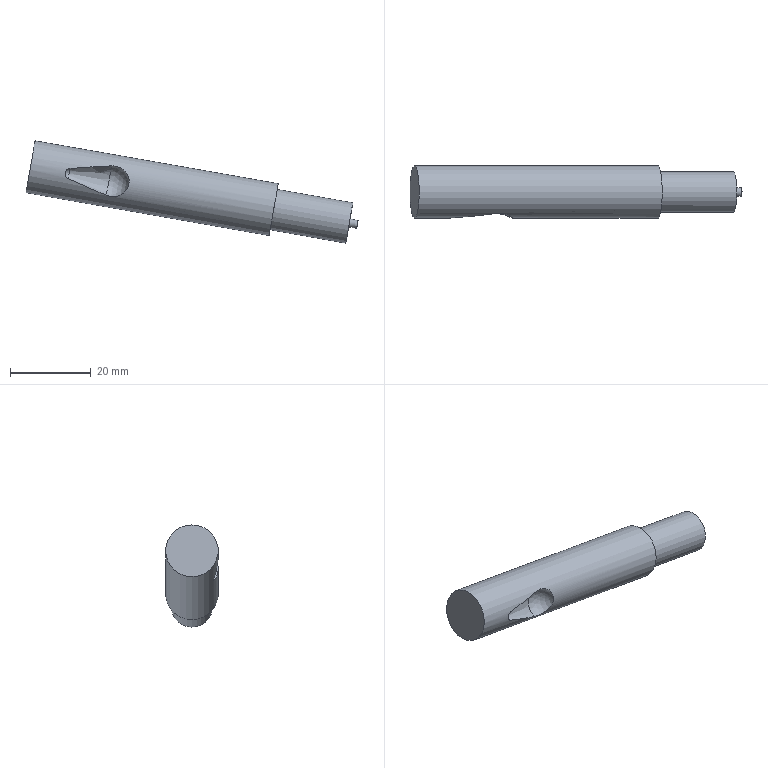Part | NX | features solid 2 | 1 solid | 10 faces | volume 9441 mm3 | plane 4 | cylinder 3 | sphere 2 | cone 1 | commonest cylinder face diameters 2 x1 10.1 x1 13 x1
STEP:
#1=CARTESIAN_POINT('',(396.16,145.871,8.418));
#2=VERTEX_POINT('',#1);
#3=CARTESIAN_POINT('',(395.283,145.871,3.444));
#4=DIRECTION('',(0.9848,0.,-0.1736));
#5=DIRECTION('',(0.1736,0.,0.9848));
#6=AXIS2_PLACEMENT_3D('',#3,#4,#5);
#7=CIRCLE('',#6,5.05);
#8=EDGE_CURVE('',#2,#2,#7,.T.);
#9=ORIENTED_EDGE('',*,*,#8,.T.);
#10=EDGE_LOOP('',(#9));
#11=FACE_BOUND('',#10,.T.);
#12=CARTESIAN_POINT('',(395.456,145.871,4.429));
#13=VERTEX_POINT('',#12);
#14=CARTESIAN_POINT('',(395.283,145.871,3.444));
#15=DIRECTION('',(0.9848,0.,-0.1736));
#16=DIRECTION('',(0.1736,0.,0.9848));
#17=AXIS2_PLACEMENT_3D('',#14,#15,#16);
#18=CIRCLE('',#17,1.);
#19=EDGE_CURVE('',#13,#13,#18,.F.);
#20=ORIENTED_EDGE('',*,*,#19,.T.);
#21=EDGE_LOOP('',(#20));
#22=FACE_BOUND('',#21,.T.);
#23=CARTESIAN_POINT('',(395.283,145.871,3.444));
#24=DIRECTION('',(-0.9848,0.,0.1736));
#25=DIRECTION('',(0.1736,0.,0.9848));
#26=AXIS2_PLACEMENT_3D('',#23,#24,#25);
#27=PLANE('',#26);
#28=ADVANCED_FACE('',(#11,#22),#27,.F.);
#29=CARTESIAN_POINT('',(336.508,140.525,17.562));
#30=VERTEX_POINT('',#29);
#31=CARTESIAN_POINT('',(326.241,139.499,16.923));
#32=VERTEX_POINT('',#31);
#33=CARTESIAN_POINT('',(336.508,140.525,17.562));
#34=CARTESIAN_POINT('',(333.101,140.013,17.411));
#35=CARTESIAN_POINT('',(329.675,139.671,17.179));
#36=CARTESIAN_POINT('',(326.241,139.499,16.923));
#37=B_SPLINE_CURVE_WITH_KNOTS('',3,(#33,#34,#35,#36),.UNSPECIFIED.,.F.,.F.,(4,4),(0.000000207,0.01034),.UNSPECIFIED.);
#38=EDGE_CURVE('',#30,#32,#37,.T.);
#39=ORIENTED_EDGE('',*,*,#38,.F.);
#40=CARTESIAN_POINT('',(335.224,140.525,10.28));
#41=VERTEX_POINT('',#40);
#42=CARTESIAN_POINT('',(335.224,140.525,10.28));
#43=CARTESIAN_POINT('',(336.35,140.708,9.813));
#44=CARTESIAN_POINT('',(338.335,140.377,9.801));
#45=CARTESIAN_POINT('',(340.189,139.555,11.301));
#46=CARTESIAN_POINT('',(340.929,139.279,13.019));
#47=CARTESIAN_POINT('',(340.826,139.556,14.903));
#48=CARTESIAN_POINT('',(339.907,140.159,16.431));
#49=CARTESIAN_POINT('',(338.355,140.634,17.394));
#50=CARTESIAN_POINT('',(337.117,140.617,17.589));
#51=CARTESIAN_POINT('',(336.508,140.525,17.562));
#52=B_SPLINE_CURVE_WITH_KNOTS('',3,(#42,#43,#44,#45,#46,#47,#48,#49,#50,#51),.UNSPECIFIED.,.F.,.F.,(4,1,1,1,1,1,1,4),(0.000000204,0.003647,0.005471,0.007295,0.009118,0.01094,0.01277,0.01459),.UNSPECIFIED.);
#53=EDGE_CURVE('',#41,#30,#52,.T.);
#54=ORIENTED_EDGE('',*,*,#53,.F.);
#55=CARTESIAN_POINT('',(325.795,139.499,14.393));
#56=VERTEX_POINT('',#55);
#57=CARTESIAN_POINT('',(325.795,139.499,14.393));
#58=CARTESIAN_POINT('',(328.935,139.671,12.977));
#59=CARTESIAN_POINT('',(332.073,140.013,11.588));
#60=CARTESIAN_POINT('',(335.224,140.525,10.28));
#61=B_SPLINE_CURVE_WITH_KNOTS('',3,(#57,#58,#59,#60),.UNSPECIFIED.,.F.,.F.,(4,4),(0.000000207,0.01035),.UNSPECIFIED.);
#62=EDGE_CURVE('',#56,#41,#61,.T.);
#63=ORIENTED_EDGE('',*,*,#62,.F.);
#64=CARTESIAN_POINT('',(326.241,139.499,16.923));
#65=CARTESIAN_POINT('',(325.652,139.47,16.879));
#66=CARTESIAN_POINT('',(324.613,139.272,15.907));
#67=CARTESIAN_POINT('',(325.256,139.47,14.636));
#68=CARTESIAN_POINT('',(325.795,139.499,14.393));
#69=B_SPLINE_CURVE_WITH_KNOTS('',3,(#64,#65,#66,#67,#68),.UNSPECIFIED.,.F.,.F.,(4,1,4),(0.000000204,0.00175,0.0035),.UNSPECIFIED.);
#70=EDGE_CURVE('',#32,#56,#69,.T.);
#71=ORIENTED_EDGE('',*,*,#70,.F.);
#72=EDGE_LOOP('',(#39,#54,#63,#71));
#73=FACE_BOUND('',#72,.T.);
#74=CARTESIAN_POINT('',(317.627,145.871,23.738));
#75=VERTEX_POINT('',#74);
#76=CARTESIAN_POINT('',(316.498,145.871,17.336));
#77=DIRECTION('',(0.9848,0.,-0.1736));
#78=DIRECTION('',(0.1736,0.,0.9848));
#79=AXIS2_PLACEMENT_3D('',#76,#77,#78);
#80=CIRCLE('',#79,6.5);
#81=EDGE_CURVE('',#75,#75,#80,.T.);
#82=ORIENTED_EDGE('',*,*,#81,.T.);
#83=EDGE_LOOP('',(#82));
#84=FACE_BOUND('',#83,.T.);
#85=CARTESIAN_POINT('',(377.7,145.871,13.145));
#86=VERTEX_POINT('',#85);
#87=CARTESIAN_POINT('',(376.571,145.871,6.744));
#88=DIRECTION('',(0.9848,0.,-0.1736));
#89=DIRECTION('',(0.1736,0.,0.9848));
#90=AXIS2_PLACEMENT_3D('',#87,#88,#89);
#91=CIRCLE('',#90,6.5);
#92=EDGE_CURVE('',#86,#86,#91,.T.);
#93=ORIENTED_EDGE('',*,*,#92,.F.);
#94=EDGE_LOOP('',(#93));
#95=FACE_BOUND('',#94,.T.);
#96=CARTESIAN_POINT('',(316.498,145.871,17.336));
#97=DIRECTION('',(0.9848,0.,-0.1736));
#98=DIRECTION('',(-0.1736,0.,-0.9848));
#99=AXIS2_PLACEMENT_3D('',#96,#97,#98);
#100=CYLINDRICAL_SURFACE('',#99,6.5);
#101=ADVANCED_FACE('',(#73,#84,#95),#100,.T.);
#102=ORIENTED_EDGE('',*,*,#81,.F.);
#103=EDGE_LOOP('',(#102));
#104=FACE_BOUND('',#103,.T.);
#105=CARTESIAN_POINT('',(316.498,145.871,17.336));
#106=DIRECTION('',(-0.9848,0.,0.1736));
#107=DIRECTION('',(0.1736,0.,0.9848));
#108=AXIS2_PLACEMENT_3D('',#105,#106,#107);
#109=PLANE('',#108);
#110=ADVANCED_FACE('',(#104),#109,.T.);
#111=CARTESIAN_POINT('',(377.448,145.871,11.717));
#112=VERTEX_POINT('',#111);
#113=CARTESIAN_POINT('',(376.571,145.871,6.744));
#114=DIRECTION('',(0.9848,0.,-0.1736));
#115=DIRECTION('',(0.1736,0.,0.9848));
#116=AXIS2_PLACEMENT_3D('',#113,#114,#115);
#117=CIRCLE('',#116,5.05);
#118=EDGE_CURVE('',#112,#112,#117,.T.);
#119=ORIENTED_EDGE('',*,*,#118,.F.);
#120=EDGE_LOOP('',(#119));
#121=FACE_BOUND('',#120,.T.);
#122=ORIENTED_EDGE('',*,*,#92,.T.);
#123=EDGE_LOOP('',(#122));
#124=FACE_BOUND('',#123,.T.);
#125=CARTESIAN_POINT('',(376.571,145.871,6.744));
#126=DIRECTION('',(-0.9848,0.,0.1736));
#127=DIRECTION('',(0.1736,0.,0.9848));
#128=AXIS2_PLACEMENT_3D('',#125,#126,#127);
#129=PLANE('',#128);
#130=ADVANCED_FACE('',(#121,#124),#129,.F.);
#131=ORIENTED_EDGE('',*,*,#8,.F.);
#132=EDGE_LOOP('',(#131));
#133=FACE_BOUND('',#132,.T.);
#134=ORIENTED_EDGE('',*,*,#118,.T.);
#135=EDGE_LOOP('',(#134));
#136=FACE_BOUND('',#135,.T.);
#137=CARTESIAN_POINT('',(395.283,145.871,3.444));
#138=DIRECTION('',(-0.9848,0.,0.1736));
#139=DIRECTION('',(0.1736,0.,0.9848));
#140=AXIS2_PLACEMENT_3D('',#137,#138,#139);
#141=CYLINDRICAL_SURFACE('',#140,5.05);
#142=ADVANCED_FACE('',(#133,#136),#141,.T.);
#143=CARTESIAN_POINT('',(335.866,139.371,13.921));
#144=DIRECTION('',(-0.9848,0.,0.1736));
#145=DIRECTION('',(-0.1736,0.,-0.9848));
#146=AXIS2_PLACEMENT_3D('',#143,#144,#145);
#147=CIRCLE('',#146,3.873);
#148=EDGE_CURVE('',#30,#41,#147,.T.);
#149=ORIENTED_EDGE('',*,*,#148,.T.);
#150=ORIENTED_EDGE('',*,*,#53,.T.);
#151=EDGE_LOOP('',(#149,#150));
#152=FACE_BOUND('',#151,.T.);
#153=CARTESIAN_POINT('',(336.851,139.371,13.748));
#154=DIRECTION('',(0.9848,0.,-0.1736));
#155=DIRECTION('',(-0.1736,0.,-0.9848));
#156=AXIS2_PLACEMENT_3D('',#153,#154,#155);
#157=SPHERICAL_SURFACE('',#156,4.);
#158=ADVANCED_FACE('',(#152),#157,.F.);
#159=CARTESIAN_POINT('',(326.018,139.371,15.658));
#160=DIRECTION('',(-0.9848,0.,0.1736));
#161=DIRECTION('',(-0.1736,0.,-0.9848));
#162=AXIS2_PLACEMENT_3D('',#159,#160,#161);
#163=CIRCLE('',#162,1.291);
#164=EDGE_CURVE('',#32,#56,#163,.T.);
#165=ORIENTED_EDGE('',*,*,#164,.T.);
#166=ORIENTED_EDGE('',*,*,#62,.T.);
#167=ORIENTED_EDGE('',*,*,#148,.F.);
#168=ORIENTED_EDGE('',*,*,#38,.T.);
#169=EDGE_LOOP('',(#165,#166,#167,#168));
#170=FACE_BOUND('',#169,.T.);
#171=CARTESIAN_POINT('',(335.866,139.371,13.921));
#172=DIRECTION('',(0.9848,0.,-0.1736));
#173=DIRECTION('',(-0.1736,0.,-0.9848));
#174=AXIS2_PLACEMENT_3D('',#171,#172,#173);
#175=CONICAL_SURFACE('',#174,3.873,0.2527);
#176=ADVANCED_FACE('',(#170),#175,.F.);
#177=ORIENTED_EDGE('',*,*,#164,.F.);
#178=ORIENTED_EDGE('',*,*,#70,.T.);
#179=EDGE_LOOP('',(#177,#178));
#180=FACE_BOUND('',#179,.T.);
#181=CARTESIAN_POINT('',(326.346,139.371,15.6));
#182=DIRECTION('',(0.9848,0.,-0.1736));
#183=DIRECTION('',(0.1736,0.,0.9848));
#184=AXIS2_PLACEMENT_3D('',#181,#182,#183);
#185=SPHERICAL_SURFACE('',#184,1.333);
#186=ADVANCED_FACE('',(#180),#185,.F.);
#187=ORIENTED_EDGE('',*,*,#19,.F.);
#188=EDGE_LOOP('',(#187));
#189=FACE_BOUND('',#188,.T.);
#190=CARTESIAN_POINT('',(397.426,145.871,4.082));
#191=VERTEX_POINT('',#190);
#192=CARTESIAN_POINT('',(397.252,145.871,3.097));
#193=DIRECTION('',(0.9848,0.,-0.1736));
#194=DIRECTION('',(0.1736,0.,0.9848));
#195=AXIS2_PLACEMENT_3D('',#192,#193,#194);
#196=CIRCLE('',#195,1.);
#197=EDGE_CURVE('',#191,#191,#196,.T.);
#198=ORIENTED_EDGE('',*,*,#197,.F.);
#199=EDGE_LOOP('',(#198));
#200=FACE_BOUND('',#199,.T.);
#201=CARTESIAN_POINT('',(395.283,145.871,3.444));
#202=DIRECTION('',(0.9848,0.,-0.1736));
#203=DIRECTION('',(-0.1736,0.,-0.9848));
#204=AXIS2_PLACEMENT_3D('',#201,#202,#203);
#205=CYLINDRICAL_SURFACE('',#204,1.);
#206=ADVANCED_FACE('',(#189,#200),#205,.T.);
#207=ORIENTED_EDGE('',*,*,#197,.T.);
#208=EDGE_LOOP('',(#207));
#209=FACE_BOUND('',#208,.T.);
#210=CARTESIAN_POINT('',(397.252,145.871,3.097));
#211=DIRECTION('',(-0.9848,0.,0.1736));
#212=DIRECTION('',(0.1736,0.,0.9848));
#213=AXIS2_PLACEMENT_3D('',#210,#211,#212);
#214=PLANE('',#213);
#215=ADVANCED_FACE('',(#209),#214,.F.);
#216=CLOSED_SHELL('',(#28,#101,#110,#130,#142,#158,#176,#186,#206,#215));
#217=MANIFOLD_SOLID_BREP('',#216);
#218=(LENGTH_UNIT()NAMED_UNIT(*)SI_UNIT(.MILLI.,.METRE.));
#219=UNCERTAINTY_MEASURE_WITH_UNIT(LENGTH_MEASURE(0.0508),#218,'','');
#220=(NAMED_UNIT(*)PLANE_ANGLE_UNIT()SI_UNIT($,.RADIAN.));
#221=(NAMED_UNIT(*)SI_UNIT($,.STERADIAN.)SOLID_ANGLE_UNIT());
#222=(GEOMETRIC_REPRESENTATION_CONTEXT(3)GLOBAL_UNCERTAINTY_ASSIGNED_CONTEXT((#219))GLOBAL_UNIT_ASSIGNED_CONTEXT((#218,#220,#221))REPRESENTATION_CONTEXT('',''));
#223=ADVANCED_BREP_SHAPE_REPRESENTATION('',(#217),#222);